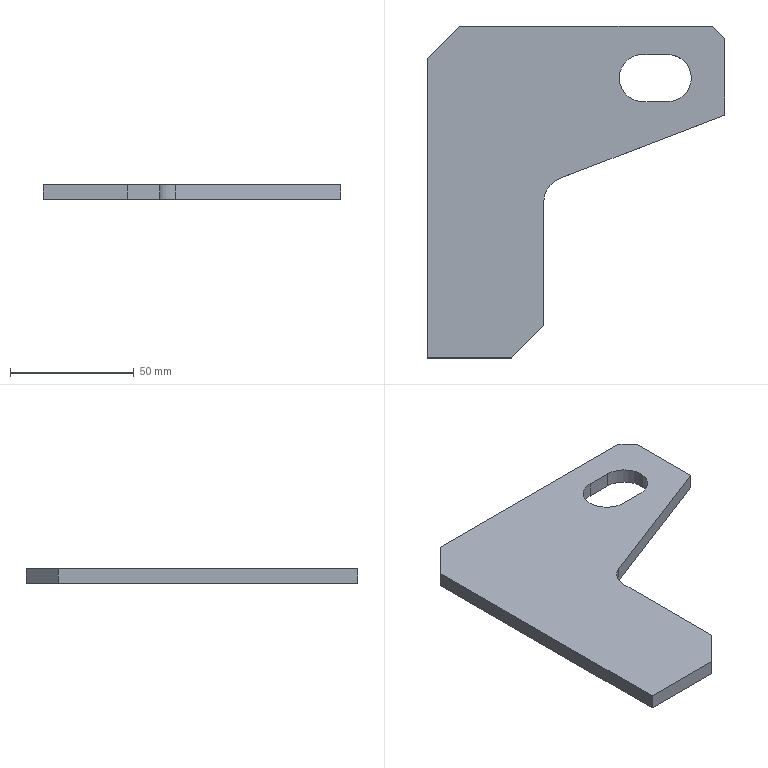Part | STEP file | 筋Plate-200×100-5-1 | 1 solid | 17 faces | box 120 x 134 x 6 mm | volume 55809 mm3 | plane 13 | cylinder 4 | commonest cylinder face diameters 19 x3 20 x1
STEP:
#1=CARTESIAN_POINT('',(0.,0.,0.));
#2=DIRECTION('',(0.,0.,1.));
#3=DIRECTION('',(1.,0.,0.));
#4=AXIS2_PLACEMENT_3D('',#1,#2,#3);
#5=CARTESIAN_POINT('',(27.,80.5,3.));
#6=VERTEX_POINT('',#5);
#7=CARTESIAN_POINT('',(27.,80.5,-3.));
#8=VERTEX_POINT('',#7);
#9=CARTESIAN_POINT('',(27.,80.5,-3.));
#10=DIRECTION('',(0.,0.,-1.));
#11=VECTOR('',#10,1.);
#12=LINE('',#9,#11);
#13=CARTESIAN_POINT('',(27.,71.,-3.));
#14=DIRECTION('',(0.,0.,-1.));
#15=DIRECTION('',(-1.,0.,0.));
#16=AXIS2_PLACEMENT_3D('',#13,#14,#15);
#17=CYLINDRICAL_SURFACE('',#16,9.5);
#18=CARTESIAN_POINT('',(1.571,0.));
#19=DIRECTION('',(0.,1.));
#20=VECTOR('',#19,1.);
#21=LINE('',#18,#20);
#22=(GEOMETRIC_REPRESENTATION_CONTEXT(2)PARAMETRIC_REPRESENTATION_CONTEXT()REPRESENTATION_CONTEXT('',''));
#23=DEFINITIONAL_REPRESENTATION('',(#21),#22);
#24=PCURVE('',#17,#23);
#25=CARTESIAN_POINT('',(37.,80.5,-3.));
#26=DIRECTION('',(0.,1.,0.));
#27=DIRECTION('',(0.,0.,1.));
#28=AXIS2_PLACEMENT_3D('',#25,#26,#27);
#29=PLANE('',#28);
#30=CARTESIAN_POINT('',(0.,-10.));
#31=DIRECTION('',(-1.,0.));
#32=VECTOR('',#31,1.);
#33=LINE('',#30,#32);
#34=(GEOMETRIC_REPRESENTATION_CONTEXT(2)PARAMETRIC_REPRESENTATION_CONTEXT()REPRESENTATION_CONTEXT('',''));
#35=DEFINITIONAL_REPRESENTATION('',(#33),#34);
#36=PCURVE('',#29,#35);
#37=SURFACE_CURVE('',#12,(#24,#36),.PCURVE_S1.);
#38=EDGE_CURVE('',#6,#8,#37,.T.);
#39=ORIENTED_EDGE('',*,*,#38,.T.);
#40=CARTESIAN_POINT('',(17.5,71.,-3.));
#41=VERTEX_POINT('',#40);
#42=CARTESIAN_POINT('',(27.,71.,-3.));
#43=DIRECTION('',(0.,0.,-1.));
#44=DIRECTION('',(-1.,0.,0.));
#45=AXIS2_PLACEMENT_3D('',#42,#43,#44);
#46=CIRCLE('',#45,9.5);
#47=CARTESIAN_POINT('',(0.,0.));
#48=DIRECTION('',(1.,0.));
#49=VECTOR('',#48,1.);
#50=LINE('',#47,#49);
#51=(GEOMETRIC_REPRESENTATION_CONTEXT(2)PARAMETRIC_REPRESENTATION_CONTEXT()REPRESENTATION_CONTEXT('',''));
#52=DEFINITIONAL_REPRESENTATION('',(#50),#51);
#53=PCURVE('',#17,#52);
#54=CARTESIAN_POINT('',(0.,0.,-3.));
#55=DIRECTION('',(0.,0.,1.));
#56=DIRECTION('',(1.,0.,0.));
#57=AXIS2_PLACEMENT_3D('',#54,#55,#56);
#58=PLANE('',#57);
#59=CARTESIAN_POINT('',(17.5,71.));
#60=CARTESIAN_POINT('',(17.5,87.454));
#61=CARTESIAN_POINT('',(31.75,79.227));
#62=CARTESIAN_POINT('',(46.,71.));
#63=CARTESIAN_POINT('',(31.75,62.773));
#64=CARTESIAN_POINT('',(17.5,54.546));
#65=CARTESIAN_POINT('',(17.5,71.));
#66=(BOUNDED_CURVE()B_SPLINE_CURVE(2,(#59,#60,#61,#62,#63,#64,#65),.UNSPECIFIED.,.T.,.F.)B_SPLINE_CURVE_WITH_KNOTS((1,2,2,2,2,1),(-2.094,0.,2.094,4.189,6.283,8.378),.UNSPECIFIED.)CURVE()GEOMETRIC_REPRESENTATION_ITEM()RATIONAL_B_SPLINE_CURVE((1.,0.5,1.,0.5,1.,0.5,1.))REPRESENTATION_ITEM(''));
#67=(GEOMETRIC_REPRESENTATION_CONTEXT(2)PARAMETRIC_REPRESENTATION_CONTEXT()REPRESENTATION_CONTEXT('',''));
#68=DEFINITIONAL_REPRESENTATION('',(#66),#67);
#69=PCURVE('',#58,#68);
#70=SURFACE_CURVE('',#46,(#53,#69),.PCURVE_S1.);
#71=EDGE_CURVE('',#41,#8,#70,.T.);
#72=ORIENTED_EDGE('',*,*,#71,.F.);
#73=CARTESIAN_POINT('',(17.5,71.,3.));
#74=VERTEX_POINT('',#73);
#75=CARTESIAN_POINT('',(17.5,71.,-3.));
#76=DIRECTION('',(0.,0.,-1.));
#77=VECTOR('',#76,1.);
#78=LINE('',#75,#77);
#79=CARTESIAN_POINT('',(0.,0.));
#80=DIRECTION('',(0.,1.));
#81=VECTOR('',#80,1.);
#82=LINE('',#79,#81);
#83=(GEOMETRIC_REPRESENTATION_CONTEXT(2)PARAMETRIC_REPRESENTATION_CONTEXT()REPRESENTATION_CONTEXT('',''));
#84=DEFINITIONAL_REPRESENTATION('',(#82),#83);
#85=PCURVE('',#17,#84);
#86=CARTESIAN_POINT('',(27.,71.,-3.));
#87=DIRECTION('',(0.,0.,-1.));
#88=DIRECTION('',(-1.,0.,0.));
#89=AXIS2_PLACEMENT_3D('',#86,#87,#88);
#90=CYLINDRICAL_SURFACE('',#89,9.5);
#91=CARTESIAN_POINT('',(6.283,0.));
#92=DIRECTION('',(0.,1.));
#93=VECTOR('',#92,1.);
#94=LINE('',#91,#93);
#95=(GEOMETRIC_REPRESENTATION_CONTEXT(2)PARAMETRIC_REPRESENTATION_CONTEXT()REPRESENTATION_CONTEXT('',''));
#96=DEFINITIONAL_REPRESENTATION('',(#94),#95);
#97=PCURVE('',#90,#96);
#98=SURFACE_CURVE('',#78,(#85,#97),.PCURVE_S1.);
#99=EDGE_CURVE('',#74,#41,#98,.T.);
#100=ORIENTED_EDGE('',*,*,#99,.F.);
#101=CARTESIAN_POINT('',(27.,71.,3.));
#102=DIRECTION('',(0.,0.,1.));
#103=DIRECTION('',(1.,0.,0.));
#104=AXIS2_PLACEMENT_3D('',#101,#102,#103);
#105=CIRCLE('',#104,9.5);
#106=CARTESIAN_POINT('',(3.142,-6.));
#107=DIRECTION('',(-1.,0.));
#108=VECTOR('',#107,1.);
#109=LINE('',#106,#108);
#110=(GEOMETRIC_REPRESENTATION_CONTEXT(2)PARAMETRIC_REPRESENTATION_CONTEXT()REPRESENTATION_CONTEXT('',''));
#111=DEFINITIONAL_REPRESENTATION('',(#109),#110);
#112=PCURVE('',#17,#111);
#113=CARTESIAN_POINT('',(0.,0.,3.));
#114=DIRECTION('',(0.,0.,1.));
#115=DIRECTION('',(1.,0.,0.));
#116=AXIS2_PLACEMENT_3D('',#113,#114,#115);
#117=PLANE('',#116);
#118=CARTESIAN_POINT('',(27.,71.));
#119=DIRECTION('',(1.,0.));
#120=AXIS2_PLACEMENT_2D('',#118,#119);
#121=CIRCLE('',#120,9.5);
#122=(GEOMETRIC_REPRESENTATION_CONTEXT(2)PARAMETRIC_REPRESENTATION_CONTEXT()REPRESENTATION_CONTEXT('',''));
#123=DEFINITIONAL_REPRESENTATION('',(#121),#122);
#124=PCURVE('',#117,#123);
#125=SURFACE_CURVE('',#105,(#112,#124),.PCURVE_S1.);
#126=EDGE_CURVE('',#6,#74,#125,.T.);
#127=ORIENTED_EDGE('',*,*,#126,.F.);
#128=EDGE_LOOP('',(#39,#72,#100,#127));
#129=FACE_BOUND('',#128,.F.);
#130=ADVANCED_FACE('',(#129),#17,.F.);
#131=CARTESIAN_POINT('',(55.,92.,-3.));
#132=VERTEX_POINT('',#131);
#133=CARTESIAN_POINT('',(-47.,92.,-3.));
#134=VERTEX_POINT('',#133);
#135=CARTESIAN_POINT('',(-60.,92.,-3.));
#136=DIRECTION('',(-1.,0.,0.));
#137=VECTOR('',#136,1.);
#138=LINE('',#135,#137);
#139=CARTESIAN_POINT('',(-60.,92.));
#140=DIRECTION('',(-1.,0.));
#141=VECTOR('',#140,1.);
#142=LINE('',#139,#141);
#143=(GEOMETRIC_REPRESENTATION_CONTEXT(2)PARAMETRIC_REPRESENTATION_CONTEXT()REPRESENTATION_CONTEXT('',''));
#144=DEFINITIONAL_REPRESENTATION('',(#142),#143);
#145=PCURVE('',#58,#144);
#146=CARTESIAN_POINT('',(-60.,92.,3.));
#147=DIRECTION('',(0.,-1.,0.));
#148=DIRECTION('',(0.,0.,-1.));
#149=AXIS2_PLACEMENT_3D('',#146,#147,#148);
#150=PLANE('',#149);
#151=CARTESIAN_POINT('',(6.,0.));
#152=DIRECTION('',(0.,-1.));
#153=VECTOR('',#152,1.);
#154=LINE('',#151,#153);
#155=(GEOMETRIC_REPRESENTATION_CONTEXT(2)PARAMETRIC_REPRESENTATION_CONTEXT()REPRESENTATION_CONTEXT('',''));
#156=DEFINITIONAL_REPRESENTATION('',(#154),#155);
#157=PCURVE('',#150,#156);
#158=SURFACE_CURVE('',#138,(#145,#157),.PCURVE_S1.);
#159=EDGE_CURVE('',#132,#134,#158,.T.);
#160=ORIENTED_EDGE('',*,*,#159,.F.);
#161=CARTESIAN_POINT('',(60.,87.,-3.));
#162=VERTEX_POINT('',#161);
#163=CARTESIAN_POINT('',(55.,92.,-3.));
#164=DIRECTION('',(0.7071,-0.7071,0.));
#165=VECTOR('',#164,1.);
#166=LINE('',#163,#165);
#167=CARTESIAN_POINT('',(55.,92.));
#168=DIRECTION('',(0.7071,-0.7071));
#169=VECTOR('',#168,1.);
#170=LINE('',#167,#169);
#171=(GEOMETRIC_REPRESENTATION_CONTEXT(2)PARAMETRIC_REPRESENTATION_CONTEXT()REPRESENTATION_CONTEXT('',''));
#172=DEFINITIONAL_REPRESENTATION('',(#170),#171);
#173=PCURVE('',#58,#172);
#174=CARTESIAN_POINT('',(55.,92.,3.));
#175=DIRECTION('',(-0.7071,-0.7071,0.));
#176=DIRECTION('',(0.,0.,-1.));
#177=AXIS2_PLACEMENT_3D('',#174,#175,#176);
#178=PLANE('',#177);
#179=CARTESIAN_POINT('',(6.,0.));
#180=DIRECTION('',(0.,1.));
#181=VECTOR('',#180,1.);
#182=LINE('',#179,#181);
#183=(GEOMETRIC_REPRESENTATION_CONTEXT(2)PARAMETRIC_REPRESENTATION_CONTEXT()REPRESENTATION_CONTEXT('',''));
#184=DEFINITIONAL_REPRESENTATION('',(#182),#183);
#185=PCURVE('',#178,#184);
#186=SURFACE_CURVE('',#166,(#173,#185),.PCURVE_S1.);
#187=EDGE_CURVE('',#132,#162,#186,.T.);
#188=ORIENTED_EDGE('',*,*,#187,.T.);
#189=CARTESIAN_POINT('',(60.,56.,-3.));
#190=VERTEX_POINT('',#189);
#191=CARTESIAN_POINT('',(60.,92.,-3.));
#192=DIRECTION('',(0.,1.,0.));
#193=VECTOR('',#192,1.);
#194=LINE('',#191,#193);
#195=CARTESIAN_POINT('',(60.,92.));
#196=DIRECTION('',(0.,1.));
#197=VECTOR('',#196,1.);
#198=LINE('',#195,#197);
#199=(GEOMETRIC_REPRESENTATION_CONTEXT(2)PARAMETRIC_REPRESENTATION_CONTEXT()REPRESENTATION_CONTEXT('',''));
#200=DEFINITIONAL_REPRESENTATION('',(#198),#199);
#201=PCURVE('',#58,#200);
#202=CARTESIAN_POINT('',(60.,92.,3.));
#203=DIRECTION('',(-1.,0.,0.));
#204=DIRECTION('',(0.,-1.,0.));
#205=AXIS2_PLACEMENT_3D('',#202,#203,#204);
#206=PLANE('',#205);
#207=CARTESIAN_POINT('',(0.,-6.));
#208=DIRECTION('',(-1.,0.));
#209=VECTOR('',#208,1.);
#210=LINE('',#207,#209);
#211=(GEOMETRIC_REPRESENTATION_CONTEXT(2)PARAMETRIC_REPRESENTATION_CONTEXT()REPRESENTATION_CONTEXT('',''));
#212=DEFINITIONAL_REPRESENTATION('',(#210),#211);
#213=PCURVE('',#206,#212);
#214=SURFACE_CURVE('',#194,(#201,#213),.PCURVE_S1.);
#215=EDGE_CURVE('',#190,#162,#214,.T.);
#216=ORIENTED_EDGE('',*,*,#215,.F.);
#217=CARTESIAN_POINT('',(-6.581,30.462,-3.));
#218=VERTEX_POINT('',#217);
#219=CARTESIAN_POINT('',(60.,56.,-3.));
#220=DIRECTION('',(-0.9337,-0.3581,0.));
#221=VECTOR('',#220,1.);
#222=LINE('',#219,#221);
#223=CARTESIAN_POINT('',(60.,56.));
#224=DIRECTION('',(-0.9337,-0.3581));
#225=VECTOR('',#224,1.);
#226=LINE('',#223,#225);
#227=(GEOMETRIC_REPRESENTATION_CONTEXT(2)PARAMETRIC_REPRESENTATION_CONTEXT()REPRESENTATION_CONTEXT('',''));
#228=DEFINITIONAL_REPRESENTATION('',(#226),#227);
#229=PCURVE('',#58,#228);
#230=CARTESIAN_POINT('',(60.,56.,-3.));
#231=DIRECTION('',(-0.3581,0.9337,0.));
#232=DIRECTION('',(-0.9337,-0.3581,0.));
#233=AXIS2_PLACEMENT_3D('',#230,#231,#232);
#234=PLANE('',#233);
#235=CARTESIAN_POINT('',(0.,0.));
#236=DIRECTION('',(1.,0.));
#237=VECTOR('',#236,1.);
#238=LINE('',#235,#237);
#239=(GEOMETRIC_REPRESENTATION_CONTEXT(2)PARAMETRIC_REPRESENTATION_CONTEXT()REPRESENTATION_CONTEXT('',''));
#240=DEFINITIONAL_REPRESENTATION('',(#238),#239);
#241=PCURVE('',#234,#240);
#242=SURFACE_CURVE('',#222,(#229,#241),.PCURVE_S1.);
#243=EDGE_CURVE('',#190,#218,#242,.T.);
#244=ORIENTED_EDGE('',*,*,#243,.T.);
#245=CARTESIAN_POINT('',(-13.,21.125,-3.));
#246=VERTEX_POINT('',#245);
#247=CARTESIAN_POINT('',(-3.,21.125,-3.));
#248=DIRECTION('',(0.,0.,1.));
#249=DIRECTION('',(1.,0.,0.));
#250=AXIS2_PLACEMENT_3D('',#247,#248,#249);
#251=CIRCLE('',#250,10.);
#252=CARTESIAN_POINT('',(-3.,21.125));
#253=DIRECTION('',(1.,0.));
#254=AXIS2_PLACEMENT_2D('',#252,#253);
#255=CIRCLE('',#254,10.);
#256=(GEOMETRIC_REPRESENTATION_CONTEXT(2)PARAMETRIC_REPRESENTATION_CONTEXT()REPRESENTATION_CONTEXT('',''));
#257=DEFINITIONAL_REPRESENTATION('',(#255),#256);
#258=PCURVE('',#58,#257);
#259=CARTESIAN_POINT('',(-3.,21.125,-3.));
#260=DIRECTION('',(0.,0.,-1.));
#261=DIRECTION('',(-1.,0.,0.));
#262=AXIS2_PLACEMENT_3D('',#259,#260,#261);
#263=CYLINDRICAL_SURFACE('',#262,10.);
#264=CARTESIAN_POINT('',(3.142,0.));
#265=DIRECTION('',(-1.,0.));
#266=VECTOR('',#265,1.);
#267=LINE('',#264,#266);
#268=(GEOMETRIC_REPRESENTATION_CONTEXT(2)PARAMETRIC_REPRESENTATION_CONTEXT()REPRESENTATION_CONTEXT('',''));
#269=DEFINITIONAL_REPRESENTATION('',(#267),#268);
#270=PCURVE('',#263,#269);
#271=SURFACE_CURVE('',#251,(#258,#270),.PCURVE_S1.);
#272=EDGE_CURVE('',#218,#246,#271,.T.);
#273=ORIENTED_EDGE('',*,*,#272,.T.);
#274=CARTESIAN_POINT('',(-13.,-29.,-3.));
#275=VERTEX_POINT('',#274);
#276=CARTESIAN_POINT('',(-13.,-92.,-3.));
#277=DIRECTION('',(0.,-1.,0.));
#278=VECTOR('',#277,1.);
#279=LINE('',#276,#278);
#280=CARTESIAN_POINT('',(-13.,-92.));
#281=DIRECTION('',(0.,-1.));
#282=VECTOR('',#281,1.);
#283=LINE('',#280,#282);
#284=(GEOMETRIC_REPRESENTATION_CONTEXT(2)PARAMETRIC_REPRESENTATION_CONTEXT()REPRESENTATION_CONTEXT('',''));
#285=DEFINITIONAL_REPRESENTATION('',(#283),#284);
#286=PCURVE('',#58,#285);
#287=CARTESIAN_POINT('',(-13.,-92.,-3.));
#288=DIRECTION('',(-1.,0.,0.));
#289=DIRECTION('',(0.,-1.,0.));
#290=AXIS2_PLACEMENT_3D('',#287,#288,#289);
#291=PLANE('',#290);
#292=CARTESIAN_POINT('',(0.,0.));
#293=DIRECTION('',(1.,0.));
#294=VECTOR('',#293,1.);
#295=LINE('',#292,#294);
#296=(GEOMETRIC_REPRESENTATION_CONTEXT(2)PARAMETRIC_REPRESENTATION_CONTEXT()REPRESENTATION_CONTEXT('',''));
#297=DEFINITIONAL_REPRESENTATION('',(#295),#296);
#298=PCURVE('',#291,#297);
#299=SURFACE_CURVE('',#279,(#286,#298),.PCURVE_S1.);
#300=EDGE_CURVE('',#246,#275,#299,.T.);
#301=ORIENTED_EDGE('',*,*,#300,.T.);
#302=CARTESIAN_POINT('',(-26.,-42.,-3.));
#303=VERTEX_POINT('',#302);
#304=CARTESIAN_POINT('',(-26.,-42.,-3.));
#305=DIRECTION('',(-0.7071,-0.7071,0.));
#306=VECTOR('',#305,1.);
#307=LINE('',#304,#306);
#308=CARTESIAN_POINT('',(-26.,-42.));
#309=DIRECTION('',(-0.7071,-0.7071));
#310=VECTOR('',#309,1.);
#311=LINE('',#308,#310);
#312=(GEOMETRIC_REPRESENTATION_CONTEXT(2)PARAMETRIC_REPRESENTATION_CONTEXT()REPRESENTATION_CONTEXT('',''));
#313=DEFINITIONAL_REPRESENTATION('',(#311),#312);
#314=PCURVE('',#58,#313);
#315=CARTESIAN_POINT('',(-26.,-42.,3.));
#316=DIRECTION('',(-0.7071,0.7071,0.));
#317=DIRECTION('',(0.,0.,1.));
#318=AXIS2_PLACEMENT_3D('',#315,#316,#317);
#319=PLANE('',#318);
#320=CARTESIAN_POINT('',(-6.,0.));
#321=DIRECTION('',(0.,-1.));
#322=VECTOR('',#321,1.);
#323=LINE('',#320,#322);
#324=(GEOMETRIC_REPRESENTATION_CONTEXT(2)PARAMETRIC_REPRESENTATION_CONTEXT()REPRESENTATION_CONTEXT('',''));
#325=DEFINITIONAL_REPRESENTATION('',(#323),#324);
#326=PCURVE('',#319,#325);
#327=SURFACE_CURVE('',#307,(#314,#326),.PCURVE_S1.);
#328=EDGE_CURVE('',#275,#303,#327,.T.);
#329=ORIENTED_EDGE('',*,*,#328,.T.);
#330=CARTESIAN_POINT('',(-60.,-42.,-3.));
#331=VERTEX_POINT('',#330);
#332=CARTESIAN_POINT('',(-60.,-42.,-3.));
#333=DIRECTION('',(1.,0.,0.));
#334=VECTOR('',#333,1.);
#335=LINE('',#332,#334);
#336=CARTESIAN_POINT('',(-60.,-42.));
#337=DIRECTION('',(1.,0.));
#338=VECTOR('',#337,1.);
#339=LINE('',#336,#338);
#340=(GEOMETRIC_REPRESENTATION_CONTEXT(2)PARAMETRIC_REPRESENTATION_CONTEXT()REPRESENTATION_CONTEXT('',''));
#341=DEFINITIONAL_REPRESENTATION('',(#339),#340);
#342=PCURVE('',#58,#341);
#343=CARTESIAN_POINT('',(-60.,-42.,3.));
#344=DIRECTION('',(0.,1.,0.));
#345=DIRECTION('',(0.,0.,1.));
#346=AXIS2_PLACEMENT_3D('',#343,#344,#345);
#347=PLANE('',#346);
#348=CARTESIAN_POINT('',(-6.,0.));
#349=DIRECTION('',(0.,1.));
#350=VECTOR('',#349,1.);
#351=LINE('',#348,#350);
#352=(GEOMETRIC_REPRESENTATION_CONTEXT(2)PARAMETRIC_REPRESENTATION_CONTEXT()REPRESENTATION_CONTEXT('',''));
#353=DEFINITIONAL_REPRESENTATION('',(#351),#352);
#354=PCURVE('',#347,#353);
#355=SURFACE_CURVE('',#335,(#342,#354),.PCURVE_S1.);
#356=EDGE_CURVE('',#331,#303,#355,.T.);
#357=ORIENTED_EDGE('',*,*,#356,.F.);
#358=CARTESIAN_POINT('',(-60.,79.,-3.));
#359=VERTEX_POINT('',#358);
#360=CARTESIAN_POINT('',(-60.,92.,-3.));
#361=DIRECTION('',(0.,-1.,0.));
#362=VECTOR('',#361,1.);
#363=LINE('',#360,#362);
#364=CARTESIAN_POINT('',(-60.,92.));
#365=DIRECTION('',(0.,-1.));
#366=VECTOR('',#365,1.);
#367=LINE('',#364,#366);
#368=(GEOMETRIC_REPRESENTATION_CONTEXT(2)PARAMETRIC_REPRESENTATION_CONTEXT()REPRESENTATION_CONTEXT('',''));
#369=DEFINITIONAL_REPRESENTATION('',(#367),#368);
#370=PCURVE('',#58,#369);
#371=CARTESIAN_POINT('',(-60.,92.,3.));
#372=DIRECTION('',(1.,0.,0.));
#373=DIRECTION('',(0.,1.,0.));
#374=AXIS2_PLACEMENT_3D('',#371,#372,#373);
#375=PLANE('',#374);
#376=CARTESIAN_POINT('',(0.,-6.));
#377=DIRECTION('',(-1.,0.));
#378=VECTOR('',#377,1.);
#379=LINE('',#376,#378);
#380=(GEOMETRIC_REPRESENTATION_CONTEXT(2)PARAMETRIC_REPRESENTATION_CONTEXT()REPRESENTATION_CONTEXT('',''));
#381=DEFINITIONAL_REPRESENTATION('',(#379),#380);
#382=PCURVE('',#375,#381);
#383=SURFACE_CURVE('',#363,(#370,#382),.PCURVE_S1.);
#384=EDGE_CURVE('',#359,#331,#383,.T.);
#385=ORIENTED_EDGE('',*,*,#384,.F.);
#386=CARTESIAN_POINT('',(-60.,79.,-3.));
#387=DIRECTION('',(0.7071,0.7071,0.));
#388=VECTOR('',#387,1.);
#389=LINE('',#386,#388);
#390=CARTESIAN_POINT('',(-60.,79.));
#391=DIRECTION('',(0.7071,0.7071));
#392=VECTOR('',#391,1.);
#393=LINE('',#390,#392);
#394=(GEOMETRIC_REPRESENTATION_CONTEXT(2)PARAMETRIC_REPRESENTATION_CONTEXT()REPRESENTATION_CONTEXT('',''));
#395=DEFINITIONAL_REPRESENTATION('',(#393),#394);
#396=PCURVE('',#58,#395);
#397=CARTESIAN_POINT('',(-60.,79.,3.));
#398=DIRECTION('',(0.7071,-0.7071,0.));
#399=DIRECTION('',(0.,0.,-1.));
#400=AXIS2_PLACEMENT_3D('',#397,#398,#399);
#401=PLANE('',#400);
#402=CARTESIAN_POINT('',(6.,0.));
#403=DIRECTION('',(0.,1.));
#404=VECTOR('',#403,1.);
#405=LINE('',#402,#404);
#406=(GEOMETRIC_REPRESENTATION_CONTEXT(2)PARAMETRIC_REPRESENTATION_CONTEXT()REPRESENTATION_CONTEXT('',''));
#407=DEFINITIONAL_REPRESENTATION('',(#405),#406);
#408=PCURVE('',#401,#407);
#409=SURFACE_CURVE('',#389,(#396,#408),.PCURVE_S1.);
#410=EDGE_CURVE('',#359,#134,#409,.T.);
#411=ORIENTED_EDGE('',*,*,#410,.T.);
#412=EDGE_LOOP('',(#160,#188,#216,#244,#273,#301,#329,#357,#385,#411));
#413=FACE_BOUND('',#412,.T.);
#414=CARTESIAN_POINT('',(37.,80.5,-3.));
#415=VERTEX_POINT('',#414);
#416=CARTESIAN_POINT('',(37.,61.5,-3.));
#417=VERTEX_POINT('',#416);
#418=CARTESIAN_POINT('',(37.,71.,-3.));
#419=DIRECTION('',(0.,0.,-1.));
#420=DIRECTION('',(-1.,0.,0.));
#421=AXIS2_PLACEMENT_3D('',#418,#419,#420);
#422=CIRCLE('',#421,9.5);
#423=CARTESIAN_POINT('',(27.5,71.));
#424=CARTESIAN_POINT('',(27.5,87.454));
#425=CARTESIAN_POINT('',(41.75,79.227));
#426=CARTESIAN_POINT('',(56.,71.));
#427=CARTESIAN_POINT('',(41.75,62.773));
#428=CARTESIAN_POINT('',(27.5,54.546));
#429=CARTESIAN_POINT('',(27.5,71.));
#430=(BOUNDED_CURVE()B_SPLINE_CURVE(2,(#423,#424,#425,#426,#427,#428,#429),.UNSPECIFIED.,.T.,.F.)B_SPLINE_CURVE_WITH_KNOTS((1,2,2,2,2,1),(-2.094,0.,2.094,4.189,6.283,8.378),.UNSPECIFIED.)CURVE()GEOMETRIC_REPRESENTATION_ITEM()RATIONAL_B_SPLINE_CURVE((1.,0.5,1.,0.5,1.,0.5,1.))REPRESENTATION_ITEM(''));
#431=(GEOMETRIC_REPRESENTATION_CONTEXT(2)PARAMETRIC_REPRESENTATION_CONTEXT()REPRESENTATION_CONTEXT('',''));
#432=DEFINITIONAL_REPRESENTATION('',(#430),#431);
#433=PCURVE('',#58,#432);
#434=CARTESIAN_POINT('',(37.,71.,-3.));
#435=DIRECTION('',(0.,0.,-1.));
#436=DIRECTION('',(-1.,0.,0.));
#437=AXIS2_PLACEMENT_3D('',#434,#435,#436);
#438=CYLINDRICAL_SURFACE('',#437,9.5);
#439=CARTESIAN_POINT('',(0.,0.));
#440=DIRECTION('',(1.,0.));
#441=VECTOR('',#440,1.);
#442=LINE('',#439,#441);
#443=(GEOMETRIC_REPRESENTATION_CONTEXT(2)PARAMETRIC_REPRESENTATION_CONTEXT()REPRESENTATION_CONTEXT('',''));
#444=DEFINITIONAL_REPRESENTATION('',(#442),#443);
#445=PCURVE('',#438,#444);
#446=SURFACE_CURVE('',#422,(#433,#445),.PCURVE_S1.);
#447=EDGE_CURVE('',#415,#417,#446,.T.);
#448=ORIENTED_EDGE('',*,*,#447,.F.);
#449=CARTESIAN_POINT('',(37.,80.5,-3.));
#450=DIRECTION('',(-1.,0.,0.));
#451=VECTOR('',#450,1.);
#452=LINE('',#449,#451);
#453=CARTESIAN_POINT('',(37.,80.5));
#454=DIRECTION('',(-1.,0.));
#455=VECTOR('',#454,1.);
#456=LINE('',#453,#455);
#457=(GEOMETRIC_REPRESENTATION_CONTEXT(2)PARAMETRIC_REPRESENTATION_CONTEXT()REPRESENTATION_CONTEXT('',''));
#458=DEFINITIONAL_REPRESENTATION('',(#456),#457);
#459=PCURVE('',#58,#458);
#460=CARTESIAN_POINT('',(0.,0.));
#461=DIRECTION('',(0.,-1.));
#462=VECTOR('',#461,1.);
#463=LINE('',#460,#462);
#464=(GEOMETRIC_REPRESENTATION_CONTEXT(2)PARAMETRIC_REPRESENTATION_CONTEXT()REPRESENTATION_CONTEXT('',''));
#465=DEFINITIONAL_REPRESENTATION('',(#463),#464);
#466=PCURVE('',#29,#465);
#467=SURFACE_CURVE('',#452,(#459,#466),.PCURVE_S1.);
#468=EDGE_CURVE('',#415,#8,#467,.T.);
#469=ORIENTED_EDGE('',*,*,#468,.T.);
#470=ORIENTED_EDGE('',*,*,#71,.F.);
#471=CARTESIAN_POINT('',(27.,61.5,-3.));
#472=VERTEX_POINT('',#471);
#473=CARTESIAN_POINT('',(27.,71.,-3.));
#474=DIRECTION('',(0.,0.,-1.));
#475=DIRECTION('',(-1.,0.,0.));
#476=AXIS2_PLACEMENT_3D('',#473,#474,#475);
#477=CIRCLE('',#476,9.5);
#478=CARTESIAN_POINT('',(17.5,71.));
#479=CARTESIAN_POINT('',(17.5,87.454));
#480=CARTESIAN_POINT('',(31.75,79.227));
#481=CARTESIAN_POINT('',(46.,71.));
#482=CARTESIAN_POINT('',(31.75,62.773));
#483=CARTESIAN_POINT('',(17.5,54.546));
#484=CARTESIAN_POINT('',(17.5,71.));
#485=(BOUNDED_CURVE()B_SPLINE_CURVE(2,(#478,#479,#480,#481,#482,#483,#484),.UNSPECIFIED.,.T.,.F.)B_SPLINE_CURVE_WITH_KNOTS((1,2,2,2,2,1),(-2.094,0.,2.094,4.189,6.283,8.378),.UNSPECIFIED.)CURVE()GEOMETRIC_REPRESENTATION_ITEM()RATIONAL_B_SPLINE_CURVE((1.,0.5,1.,0.5,1.,0.5,1.))REPRESENTATION_ITEM(''));
#486=(GEOMETRIC_REPRESENTATION_CONTEXT(2)PARAMETRIC_REPRESENTATION_CONTEXT()REPRESENTATION_CONTEXT('',''));
#487=DEFINITIONAL_REPRESENTATION('',(#485),#486);
#488=PCURVE('',#58,#487);
#489=CARTESIAN_POINT('',(0.,0.));
#490=DIRECTION('',(1.,0.));
#491=VECTOR('',#490,1.);
#492=LINE('',#489,#491);
#493=(GEOMETRIC_REPRESENTATION_CONTEXT(2)PARAMETRIC_REPRESENTATION_CONTEXT()REPRESENTATION_CONTEXT('',''));
#494=DEFINITIONAL_REPRESENTATION('',(#492),#493);
#495=PCURVE('',#90,#494);
#496=SURFACE_CURVE('',#477,(#488,#495),.PCURVE_S1.);
#497=EDGE_CURVE('',#472,#41,#496,.T.);
#498=ORIENTED_EDGE('',*,*,#497,.F.);
#499=CARTESIAN_POINT('',(37.,61.5,-3.));
#500=DIRECTION('',(-1.,0.,0.));
#501=VECTOR('',#500,1.);
#502=LINE('',#499,#501);
#503=CARTESIAN_POINT('',(37.,61.5));
#504=DIRECTION('',(-1.,0.));
#505=VECTOR('',#504,1.);
#506=LINE('',#503,#505);
#507=(GEOMETRIC_REPRESENTATION_CONTEXT(2)PARAMETRIC_REPRESENTATION_CONTEXT()REPRESENTATION_CONTEXT('',''));
#508=DEFINITIONAL_REPRESENTATION('',(#506),#507);
#509=PCURVE('',#58,#508);
#510=CARTESIAN_POINT('',(37.,61.5,-3.));
#511=DIRECTION('',(0.,-1.,0.));
#512=DIRECTION('',(0.,0.,-1.));
#513=AXIS2_PLACEMENT_3D('',#510,#511,#512);
#514=PLANE('',#513);
#515=CARTESIAN_POINT('',(0.,0.));
#516=DIRECTION('',(0.,-1.));
#517=VECTOR('',#516,1.);
#518=LINE('',#515,#517);
#519=(GEOMETRIC_REPRESENTATION_CONTEXT(2)PARAMETRIC_REPRESENTATION_CONTEXT()REPRESENTATION_CONTEXT('',''));
#520=DEFINITIONAL_REPRESENTATION('',(#518),#519);
#521=PCURVE('',#514,#520);
#522=SURFACE_CURVE('',#502,(#509,#521),.PCURVE_S1.);
#523=EDGE_CURVE('',#417,#472,#522,.T.);
#524=ORIENTED_EDGE('',*,*,#523,.F.);
#525=EDGE_LOOP('',(#448,#469,#470,#498,#524));
#526=FACE_BOUND('',#525,.T.);
#527=ADVANCED_FACE('',(#413,#526),#58,.F.);
#528=ORIENTED_EDGE('',*,*,#215,.T.);
#529=CARTESIAN_POINT('',(60.,87.,3.));
#530=VERTEX_POINT('',#529);
#531=CARTESIAN_POINT('',(60.,87.,3.));
#532=DIRECTION('',(0.,0.,1.));
#533=VECTOR('',#532,1.);
#534=LINE('',#531,#533);
#535=CARTESIAN_POINT('',(5.,0.));
#536=DIRECTION('',(0.,1.));
#537=VECTOR('',#536,1.);
#538=LINE('',#535,#537);
#539=(GEOMETRIC_REPRESENTATION_CONTEXT(2)PARAMETRIC_REPRESENTATION_CONTEXT()REPRESENTATION_CONTEXT('',''));
#540=DEFINITIONAL_REPRESENTATION('',(#538),#539);
#541=PCURVE('',#206,#540);
#542=CARTESIAN_POINT('',(0.,7.071));
#543=DIRECTION('',(-1.,0.));
#544=VECTOR('',#543,1.);
#545=LINE('',#542,#544);
#546=(GEOMETRIC_REPRESENTATION_CONTEXT(2)PARAMETRIC_REPRESENTATION_CONTEXT()REPRESENTATION_CONTEXT('',''));
#547=DEFINITIONAL_REPRESENTATION('',(#545),#546);
#548=PCURVE('',#178,#547);
#549=SURFACE_CURVE('',#534,(#541,#548),.PCURVE_S1.);
#550=EDGE_CURVE('',#162,#530,#549,.T.);
#551=ORIENTED_EDGE('',*,*,#550,.T.);
#552=CARTESIAN_POINT('',(60.,56.,3.));
#553=VERTEX_POINT('',#552);
#554=CARTESIAN_POINT('',(60.,92.,3.));
#555=DIRECTION('',(0.,1.,0.));
#556=VECTOR('',#555,1.);
#557=LINE('',#554,#556);
#558=CARTESIAN_POINT('',(0.,0.));
#559=DIRECTION('',(-1.,0.));
#560=VECTOR('',#559,1.);
#561=LINE('',#558,#560);
#562=(GEOMETRIC_REPRESENTATION_CONTEXT(2)PARAMETRIC_REPRESENTATION_CONTEXT()REPRESENTATION_CONTEXT('',''));
#563=DEFINITIONAL_REPRESENTATION('',(#561),#562);
#564=PCURVE('',#206,#563);
#565=CARTESIAN_POINT('',(60.,92.));
#566=DIRECTION('',(0.,1.));
#567=VECTOR('',#566,1.);
#568=LINE('',#565,#567);
#569=(GEOMETRIC_REPRESENTATION_CONTEXT(2)PARAMETRIC_REPRESENTATION_CONTEXT()REPRESENTATION_CONTEXT('',''));
#570=DEFINITIONAL_REPRESENTATION('',(#568),#569);
#571=PCURVE('',#117,#570);
#572=SURFACE_CURVE('',#557,(#564,#571),.PCURVE_S1.);
#573=EDGE_CURVE('',#553,#530,#572,.T.);
#574=ORIENTED_EDGE('',*,*,#573,.F.);
#575=CARTESIAN_POINT('',(60.,56.,-3.));
#576=DIRECTION('',(0.,0.,1.));
#577=VECTOR('',#576,1.);
#578=LINE('',#575,#577);
#579=CARTESIAN_POINT('',(36.,-6.));
#580=DIRECTION('',(0.,1.));
#581=VECTOR('',#580,1.);
#582=LINE('',#579,#581);
#583=(GEOMETRIC_REPRESENTATION_CONTEXT(2)PARAMETRIC_REPRESENTATION_CONTEXT()REPRESENTATION_CONTEXT('',''));
#584=DEFINITIONAL_REPRESENTATION('',(#582),#583);
#585=PCURVE('',#206,#584);
#586=CARTESIAN_POINT('',(0.,0.));
#587=DIRECTION('',(0.,1.));
#588=VECTOR('',#587,1.);
#589=LINE('',#586,#588);
#590=(GEOMETRIC_REPRESENTATION_CONTEXT(2)PARAMETRIC_REPRESENTATION_CONTEXT()REPRESENTATION_CONTEXT('',''));
#591=DEFINITIONAL_REPRESENTATION('',(#589),#590);
#592=PCURVE('',#234,#591);
#593=SURFACE_CURVE('',#578,(#585,#592),.PCURVE_S1.);
#594=EDGE_CURVE('',#190,#553,#593,.T.);
#595=ORIENTED_EDGE('',*,*,#594,.F.);
#596=EDGE_LOOP('',(#528,#551,#574,#595));
#597=FACE_BOUND('',#596,.T.);
#598=ADVANCED_FACE('',(#597),#206,.F.);
#599=CARTESIAN_POINT('',(55.,92.,3.));
#600=VERTEX_POINT('',#599);
#601=CARTESIAN_POINT('',(-47.,92.,3.));
#602=VERTEX_POINT('',#601);
#603=CARTESIAN_POINT('',(-60.,92.,3.));
#604=DIRECTION('',(-1.,0.,0.));
#605=VECTOR('',#604,1.);
#606=LINE('',#603,#605);
#607=CARTESIAN_POINT('',(0.,0.));
#608=DIRECTION('',(0.,-1.));
#609=VECTOR('',#608,1.);
#610=LINE('',#607,#609);
#611=(GEOMETRIC_REPRESENTATION_CONTEXT(2)PARAMETRIC_REPRESENTATION_CONTEXT()REPRESENTATION_CONTEXT('',''));
#612=DEFINITIONAL_REPRESENTATION('',(#610),#611);
#613=PCURVE('',#150,#612);
#614=CARTESIAN_POINT('',(-60.,92.));
#615=DIRECTION('',(-1.,0.));
#616=VECTOR('',#615,1.);
#617=LINE('',#614,#616);
#618=(GEOMETRIC_REPRESENTATION_CONTEXT(2)PARAMETRIC_REPRESENTATION_CONTEXT()REPRESENTATION_CONTEXT('',''));
#619=DEFINITIONAL_REPRESENTATION('',(#617),#618);
#620=PCURVE('',#117,#619);
#621=SURFACE_CURVE('',#606,(#613,#620),.PCURVE_S1.);
#622=EDGE_CURVE('',#600,#602,#621,.T.);
#623=ORIENTED_EDGE('',*,*,#622,.F.);
#624=CARTESIAN_POINT('',(55.,92.,3.));
#625=DIRECTION('',(0.,0.,-1.));
#626=VECTOR('',#625,1.);
#627=LINE('',#624,#626);
#628=CARTESIAN_POINT('',(0.,115.));
#629=DIRECTION('',(1.,0.));
#630=VECTOR('',#629,1.);
#631=LINE('',#628,#630);
#632=(GEOMETRIC_REPRESENTATION_CONTEXT(2)PARAMETRIC_REPRESENTATION_CONTEXT()REPRESENTATION_CONTEXT('',''));
#633=DEFINITIONAL_REPRESENTATION('',(#631),#632);
#634=PCURVE('',#150,#633);
#635=CARTESIAN_POINT('',(0.,0.));
#636=DIRECTION('',(1.,0.));
#637=VECTOR('',#636,1.);
#638=LINE('',#635,#637);
#639=(GEOMETRIC_REPRESENTATION_CONTEXT(2)PARAMETRIC_REPRESENTATION_CONTEXT()REPRESENTATION_CONTEXT('',''));
#640=DEFINITIONAL_REPRESENTATION('',(#638),#639);
#641=PCURVE('',#178,#640);
#642=SURFACE_CURVE('',#627,(#634,#641),.PCURVE_S1.);
#643=EDGE_CURVE('',#600,#132,#642,.T.);
#644=ORIENTED_EDGE('',*,*,#643,.T.);
#645=ORIENTED_EDGE('',*,*,#159,.T.);
#646=CARTESIAN_POINT('',(-47.,92.,3.));
#647=DIRECTION('',(0.,0.,1.));
#648=VECTOR('',#647,1.);
#649=LINE('',#646,#648);
#650=CARTESIAN_POINT('',(0.,13.));
#651=DIRECTION('',(-1.,0.));
#652=VECTOR('',#651,1.);
#653=LINE('',#650,#652);
#654=(GEOMETRIC_REPRESENTATION_CONTEXT(2)PARAMETRIC_REPRESENTATION_CONTEXT()REPRESENTATION_CONTEXT('',''));
#655=DEFINITIONAL_REPRESENTATION('',(#653),#654);
#656=PCURVE('',#150,#655);
#657=CARTESIAN_POINT('',(0.,18.385));
#658=DIRECTION('',(-1.,0.));
#659=VECTOR('',#658,1.);
#660=LINE('',#657,#659);
#661=(GEOMETRIC_REPRESENTATION_CONTEXT(2)PARAMETRIC_REPRESENTATION_CONTEXT()REPRESENTATION_CONTEXT('',''));
#662=DEFINITIONAL_REPRESENTATION('',(#660),#661);
#663=PCURVE('',#401,#662);
#664=SURFACE_CURVE('',#649,(#656,#663),.PCURVE_S1.);
#665=EDGE_CURVE('',#134,#602,#664,.T.);
#666=ORIENTED_EDGE('',*,*,#665,.T.);
#667=EDGE_LOOP('',(#623,#644,#645,#666));
#668=FACE_BOUND('',#667,.T.);
#669=ADVANCED_FACE('',(#668),#150,.F.);
#670=CARTESIAN_POINT('',(-60.,79.,3.));
#671=VERTEX_POINT('',#670);
#672=CARTESIAN_POINT('',(-60.,-42.,3.));
#673=VERTEX_POINT('',#672);
#674=CARTESIAN_POINT('',(-60.,92.,3.));
#675=DIRECTION('',(0.,-1.,0.));
#676=VECTOR('',#675,1.);
#677=LINE('',#674,#676);
#678=CARTESIAN_POINT('',(0.,0.));
#679=DIRECTION('',(-1.,0.));
#680=VECTOR('',#679,1.);
#681=LINE('',#678,#680);
#682=(GEOMETRIC_REPRESENTATION_CONTEXT(2)PARAMETRIC_REPRESENTATION_CONTEXT()REPRESENTATION_CONTEXT('',''));
#683=DEFINITIONAL_REPRESENTATION('',(#681),#682);
#684=PCURVE('',#375,#683);
#685=CARTESIAN_POINT('',(-60.,92.));
#686=DIRECTION('',(0.,-1.));
#687=VECTOR('',#686,1.);
#688=LINE('',#685,#687);
#689=(GEOMETRIC_REPRESENTATION_CONTEXT(2)PARAMETRIC_REPRESENTATION_CONTEXT()REPRESENTATION_CONTEXT('',''));
#690=DEFINITIONAL_REPRESENTATION('',(#688),#689);
#691=PCURVE('',#117,#690);
#692=SURFACE_CURVE('',#677,(#684,#691),.PCURVE_S1.);
#693=EDGE_CURVE('',#671,#673,#692,.T.);
#694=ORIENTED_EDGE('',*,*,#693,.F.);
#695=CARTESIAN_POINT('',(-60.,79.,3.));
#696=DIRECTION('',(0.,0.,-1.));
#697=VECTOR('',#696,1.);
#698=LINE('',#695,#697);
#699=CARTESIAN_POINT('',(-13.,0.));
#700=DIRECTION('',(0.,-1.));
#701=VECTOR('',#700,1.);
#702=LINE('',#699,#701);
#703=(GEOMETRIC_REPRESENTATION_CONTEXT(2)PARAMETRIC_REPRESENTATION_CONTEXT()REPRESENTATION_CONTEXT('',''));
#704=DEFINITIONAL_REPRESENTATION('',(#702),#703);
#705=PCURVE('',#375,#704);
#706=CARTESIAN_POINT('',(0.,0.));
#707=DIRECTION('',(1.,0.));
#708=VECTOR('',#707,1.);
#709=LINE('',#706,#708);
#710=(GEOMETRIC_REPRESENTATION_CONTEXT(2)PARAMETRIC_REPRESENTATION_CONTEXT()REPRESENTATION_CONTEXT('',''));
#711=DEFINITIONAL_REPRESENTATION('',(#709),#710);
#712=PCURVE('',#401,#711);
#713=SURFACE_CURVE('',#698,(#705,#712),.PCURVE_S1.);
#714=EDGE_CURVE('',#671,#359,#713,.T.);
#715=ORIENTED_EDGE('',*,*,#714,.T.);
#716=ORIENTED_EDGE('',*,*,#384,.T.);
#717=CARTESIAN_POINT('',(-60.,-42.,3.));
#718=DIRECTION('',(0.,0.,-1.));
#719=VECTOR('',#718,1.);
#720=LINE('',#717,#719);
#721=CARTESIAN_POINT('',(-134.,0.));
#722=DIRECTION('',(0.,-1.));
#723=VECTOR('',#722,1.);
#724=LINE('',#721,#723);
#725=(GEOMETRIC_REPRESENTATION_CONTEXT(2)PARAMETRIC_REPRESENTATION_CONTEXT()REPRESENTATION_CONTEXT('',''));
#726=DEFINITIONAL_REPRESENTATION('',(#724),#725);
#727=PCURVE('',#375,#726);
#728=CARTESIAN_POINT('',(0.,0.));
#729=DIRECTION('',(-1.,0.));
#730=VECTOR('',#729,1.);
#731=LINE('',#728,#730);
#732=(GEOMETRIC_REPRESENTATION_CONTEXT(2)PARAMETRIC_REPRESENTATION_CONTEXT()REPRESENTATION_CONTEXT('',''));
#733=DEFINITIONAL_REPRESENTATION('',(#731),#732);
#734=PCURVE('',#347,#733);
#735=SURFACE_CURVE('',#720,(#727,#734),.PCURVE_S1.);
#736=EDGE_CURVE('',#673,#331,#735,.T.);
#737=ORIENTED_EDGE('',*,*,#736,.F.);
#738=EDGE_LOOP('',(#694,#715,#716,#737));
#739=FACE_BOUND('',#738,.T.);
#740=ADVANCED_FACE('',(#739),#375,.F.);
#741=ORIENTED_EDGE('',*,*,#356,.T.);
#742=CARTESIAN_POINT('',(-26.,-42.,3.));
#743=VERTEX_POINT('',#742);
#744=CARTESIAN_POINT('',(-26.,-42.,3.));
#745=DIRECTION('',(0.,0.,1.));
#746=VECTOR('',#745,1.);
#747=LINE('',#744,#746);
#748=CARTESIAN_POINT('',(0.,34.));
#749=DIRECTION('',(1.,0.));
#750=VECTOR('',#749,1.);
#751=LINE('',#748,#750);
#752=(GEOMETRIC_REPRESENTATION_CONTEXT(2)PARAMETRIC_REPRESENTATION_CONTEXT()REPRESENTATION_CONTEXT('',''));
#753=DEFINITIONAL_REPRESENTATION('',(#751),#752);
#754=PCURVE('',#347,#753);
#755=CARTESIAN_POINT('',(0.,0.));
#756=DIRECTION('',(1.,0.));
#757=VECTOR('',#756,1.);
#758=LINE('',#755,#757);
#759=(GEOMETRIC_REPRESENTATION_CONTEXT(2)PARAMETRIC_REPRESENTATION_CONTEXT()REPRESENTATION_CONTEXT('',''));
#760=DEFINITIONAL_REPRESENTATION('',(#758),#759);
#761=PCURVE('',#319,#760);
#762=SURFACE_CURVE('',#747,(#754,#761),.PCURVE_S1.);
#763=EDGE_CURVE('',#303,#743,#762,.T.);
#764=ORIENTED_EDGE('',*,*,#763,.T.);
#765=CARTESIAN_POINT('',(-60.,-42.,3.));
#766=DIRECTION('',(1.,0.,0.));
#767=VECTOR('',#766,1.);
#768=LINE('',#765,#767);
#769=CARTESIAN_POINT('',(0.,0.));
#770=DIRECTION('',(0.,1.));
#771=VECTOR('',#770,1.);
#772=LINE('',#769,#771);
#773=(GEOMETRIC_REPRESENTATION_CONTEXT(2)PARAMETRIC_REPRESENTATION_CONTEXT()REPRESENTATION_CONTEXT('',''));
#774=DEFINITIONAL_REPRESENTATION('',(#772),#773);
#775=PCURVE('',#347,#774);
#776=CARTESIAN_POINT('',(-60.,-42.));
#777=DIRECTION('',(1.,0.));
#778=VECTOR('',#777,1.);
#779=LINE('',#776,#778);
#780=(GEOMETRIC_REPRESENTATION_CONTEXT(2)PARAMETRIC_REPRESENTATION_CONTEXT()REPRESENTATION_CONTEXT('',''));
#781=DEFINITIONAL_REPRESENTATION('',(#779),#780);
#782=PCURVE('',#117,#781);
#783=SURFACE_CURVE('',#768,(#775,#782),.PCURVE_S1.);
#784=EDGE_CURVE('',#673,#743,#783,.T.);
#785=ORIENTED_EDGE('',*,*,#784,.F.);
#786=ORIENTED_EDGE('',*,*,#736,.T.);
#787=EDGE_LOOP('',(#741,#764,#785,#786));
#788=FACE_BOUND('',#787,.T.);
#789=ADVANCED_FACE('',(#788),#347,.F.);
#790=CARTESIAN_POINT('',(37.,61.5,3.));
#791=VERTEX_POINT('',#790);
#792=CARTESIAN_POINT('',(37.,80.5,3.));
#793=VERTEX_POINT('',#792);
#794=CARTESIAN_POINT('',(37.,71.,3.));
#795=DIRECTION('',(0.,0.,1.));
#796=DIRECTION('',(1.,0.,0.));
#797=AXIS2_PLACEMENT_3D('',#794,#795,#796);
#798=CIRCLE('',#797,9.5);
#799=CARTESIAN_POINT('',(37.,71.));
#800=DIRECTION('',(1.,0.));
#801=AXIS2_PLACEMENT_2D('',#799,#800);
#802=CIRCLE('',#801,9.5);
#803=(GEOMETRIC_REPRESENTATION_CONTEXT(2)PARAMETRIC_REPRESENTATION_CONTEXT()REPRESENTATION_CONTEXT('',''));
#804=DEFINITIONAL_REPRESENTATION('',(#802),#803);
#805=PCURVE('',#117,#804);
#806=CARTESIAN_POINT('',(9.425,-6.));
#807=DIRECTION('',(-1.,0.));
#808=VECTOR('',#807,1.);
#809=LINE('',#806,#808);
#810=(GEOMETRIC_REPRESENTATION_CONTEXT(2)PARAMETRIC_REPRESENTATION_CONTEXT()REPRESENTATION_CONTEXT('',''));
#811=DEFINITIONAL_REPRESENTATION('',(#809),#810);
#812=PCURVE('',#438,#811);
#813=SURFACE_CURVE('',#798,(#805,#812),.PCURVE_S1.);
#814=EDGE_CURVE('',#791,#793,#813,.T.);
#815=ORIENTED_EDGE('',*,*,#814,.F.);
#816=CARTESIAN_POINT('',(27.,61.5,3.));
#817=VERTEX_POINT('',#816);
#818=CARTESIAN_POINT('',(0.,61.5,3.));
#819=DIRECTION('',(1.,0.,0.));
#820=VECTOR('',#819,1.);
#821=LINE('',#818,#820);
#822=CARTESIAN_POINT('',(0.,61.5));
#823=DIRECTION('',(1.,0.));
#824=VECTOR('',#823,1.);
#825=LINE('',#822,#824);
#826=(GEOMETRIC_REPRESENTATION_CONTEXT(2)PARAMETRIC_REPRESENTATION_CONTEXT()REPRESENTATION_CONTEXT('',''));
#827=DEFINITIONAL_REPRESENTATION('',(#825),#826);
#828=PCURVE('',#117,#827);
#829=CARTESIAN_POINT('',(-6.,-37.));
#830=DIRECTION('',(0.,1.));
#831=VECTOR('',#830,1.);
#832=LINE('',#829,#831);
#833=(GEOMETRIC_REPRESENTATION_CONTEXT(2)PARAMETRIC_REPRESENTATION_CONTEXT()REPRESENTATION_CONTEXT('',''));
#834=DEFINITIONAL_REPRESENTATION('',(#832),#833);
#835=PCURVE('',#514,#834);
#836=SURFACE_CURVE('',#821,(#828,#835),.PCURVE_S1.);
#837=EDGE_CURVE('',#817,#791,#836,.T.);
#838=ORIENTED_EDGE('',*,*,#837,.F.);
#839=CARTESIAN_POINT('',(27.,71.,3.));
#840=DIRECTION('',(0.,0.,1.));
#841=DIRECTION('',(1.,0.,0.));
#842=AXIS2_PLACEMENT_3D('',#839,#840,#841);
#843=CIRCLE('',#842,9.5);
#844=CARTESIAN_POINT('',(27.,71.));
#845=DIRECTION('',(1.,0.));
#846=AXIS2_PLACEMENT_2D('',#844,#845);
#847=CIRCLE('',#846,9.5);
#848=(GEOMETRIC_REPRESENTATION_CONTEXT(2)PARAMETRIC_REPRESENTATION_CONTEXT()REPRESENTATION_CONTEXT('',''));
#849=DEFINITIONAL_REPRESENTATION('',(#847),#848);
#850=PCURVE('',#117,#849);
#851=CARTESIAN_POINT('',(9.425,-6.));
#852=DIRECTION('',(-1.,0.));
#853=VECTOR('',#852,1.);
#854=LINE('',#851,#853);
#855=(GEOMETRIC_REPRESENTATION_CONTEXT(2)PARAMETRIC_REPRESENTATION_CONTEXT()REPRESENTATION_CONTEXT('',''));
#856=DEFINITIONAL_REPRESENTATION('',(#854),#855);
#857=PCURVE('',#90,#856);
#858=SURFACE_CURVE('',#843,(#850,#857),.PCURVE_S1.);
#859=EDGE_CURVE('',#74,#817,#858,.T.);
#860=ORIENTED_EDGE('',*,*,#859,.F.);
#861=ORIENTED_EDGE('',*,*,#126,.F.);
#862=CARTESIAN_POINT('',(0.,80.5,3.));
#863=DIRECTION('',(-1.,0.,0.));
#864=VECTOR('',#863,1.);
#865=LINE('',#862,#864);
#866=CARTESIAN_POINT('',(0.,80.5));
#867=DIRECTION('',(-1.,0.));
#868=VECTOR('',#867,1.);
#869=LINE('',#866,#868);
#870=(GEOMETRIC_REPRESENTATION_CONTEXT(2)PARAMETRIC_REPRESENTATION_CONTEXT()REPRESENTATION_CONTEXT('',''));
#871=DEFINITIONAL_REPRESENTATION('',(#869),#870);
#872=PCURVE('',#117,#871);
#873=CARTESIAN_POINT('',(6.,-37.));
#874=DIRECTION('',(0.,-1.));
#875=VECTOR('',#874,1.);
#876=LINE('',#873,#875);
#877=(GEOMETRIC_REPRESENTATION_CONTEXT(2)PARAMETRIC_REPRESENTATION_CONTEXT()REPRESENTATION_CONTEXT('',''));
#878=DEFINITIONAL_REPRESENTATION('',(#876),#877);
#879=PCURVE('',#29,#878);
#880=SURFACE_CURVE('',#865,(#872,#879),.PCURVE_S1.);
#881=EDGE_CURVE('',#793,#6,#880,.T.);
#882=ORIENTED_EDGE('',*,*,#881,.F.);
#883=EDGE_LOOP('',(#815,#838,#860,#861,#882));
#884=FACE_BOUND('',#883,.T.);
#885=ORIENTED_EDGE('',*,*,#573,.T.);
#886=CARTESIAN_POINT('',(73.5,73.5,3.));
#887=DIRECTION('',(-0.7071,0.7071,0.));
#888=VECTOR('',#887,1.);
#889=LINE('',#886,#888);
#890=CARTESIAN_POINT('',(73.5,73.5));
#891=DIRECTION('',(-0.7071,0.7071));
#892=VECTOR('',#891,1.);
#893=LINE('',#890,#892);
#894=(GEOMETRIC_REPRESENTATION_CONTEXT(2)PARAMETRIC_REPRESENTATION_CONTEXT()REPRESENTATION_CONTEXT('',''));
#895=DEFINITIONAL_REPRESENTATION('',(#893),#894);
#896=PCURVE('',#117,#895);
#897=CARTESIAN_POINT('',(0.,26.163));
#898=DIRECTION('',(0.,-1.));
#899=VECTOR('',#898,1.);
#900=LINE('',#897,#899);
#901=(GEOMETRIC_REPRESENTATION_CONTEXT(2)PARAMETRIC_REPRESENTATION_CONTEXT()REPRESENTATION_CONTEXT('',''));
#902=DEFINITIONAL_REPRESENTATION('',(#900),#901);
#903=PCURVE('',#178,#902);
#904=SURFACE_CURVE('',#889,(#896,#903),.PCURVE_S1.);
#905=EDGE_CURVE('',#530,#600,#904,.T.);
#906=ORIENTED_EDGE('',*,*,#905,.T.);
#907=ORIENTED_EDGE('',*,*,#622,.T.);
#908=CARTESIAN_POINT('',(-69.5,69.5,3.));
#909=DIRECTION('',(-0.7071,-0.7071,0.));
#910=VECTOR('',#909,1.);
#911=LINE('',#908,#910);
#912=CARTESIAN_POINT('',(-69.5,69.5));
#913=DIRECTION('',(-0.7071,-0.7071));
#914=VECTOR('',#913,1.);
#915=LINE('',#912,#914);
#916=(GEOMETRIC_REPRESENTATION_CONTEXT(2)PARAMETRIC_REPRESENTATION_CONTEXT()REPRESENTATION_CONTEXT('',''));
#917=DEFINITIONAL_REPRESENTATION('',(#915),#916);
#918=PCURVE('',#117,#917);
#919=CARTESIAN_POINT('',(0.,-13.435));
#920=DIRECTION('',(0.,-1.));
#921=VECTOR('',#920,1.);
#922=LINE('',#919,#921);
#923=(GEOMETRIC_REPRESENTATION_CONTEXT(2)PARAMETRIC_REPRESENTATION_CONTEXT()REPRESENTATION_CONTEXT('',''));
#924=DEFINITIONAL_REPRESENTATION('',(#922),#923);
#925=PCURVE('',#401,#924);
#926=SURFACE_CURVE('',#911,(#918,#925),.PCURVE_S1.);
#927=EDGE_CURVE('',#602,#671,#926,.T.);
#928=ORIENTED_EDGE('',*,*,#927,.T.);
#929=ORIENTED_EDGE('',*,*,#693,.T.);
#930=ORIENTED_EDGE('',*,*,#784,.T.);
#931=CARTESIAN_POINT('',(-13.,-29.,3.));
#932=VERTEX_POINT('',#931);
#933=CARTESIAN_POINT('',(33.,17.,3.));
#934=DIRECTION('',(0.7071,0.7071,0.));
#935=VECTOR('',#934,1.);
#936=LINE('',#933,#935);
#937=CARTESIAN_POINT('',(33.,17.));
#938=DIRECTION('',(0.7071,0.7071));
#939=VECTOR('',#938,1.);
#940=LINE('',#937,#939);
#941=(GEOMETRIC_REPRESENTATION_CONTEXT(2)PARAMETRIC_REPRESENTATION_CONTEXT()REPRESENTATION_CONTEXT('',''));
#942=DEFINITIONAL_REPRESENTATION('',(#940),#941);
#943=PCURVE('',#117,#942);
#944=CARTESIAN_POINT('',(0.,83.439));
#945=DIRECTION('',(0.,1.));
#946=VECTOR('',#945,1.);
#947=LINE('',#944,#946);
#948=(GEOMETRIC_REPRESENTATION_CONTEXT(2)PARAMETRIC_REPRESENTATION_CONTEXT()REPRESENTATION_CONTEXT('',''));
#949=DEFINITIONAL_REPRESENTATION('',(#947),#948);
#950=PCURVE('',#319,#949);
#951=SURFACE_CURVE('',#936,(#943,#950),.PCURVE_S1.);
#952=EDGE_CURVE('',#743,#932,#951,.T.);
#953=ORIENTED_EDGE('',*,*,#952,.T.);
#954=CARTESIAN_POINT('',(-13.,21.125,3.));
#955=VERTEX_POINT('',#954);
#956=CARTESIAN_POINT('',(-13.,-92.,3.));
#957=DIRECTION('',(0.,-1.,0.));
#958=VECTOR('',#957,1.);
#959=LINE('',#956,#958);
#960=CARTESIAN_POINT('',(-13.,-92.));
#961=DIRECTION('',(0.,-1.));
#962=VECTOR('',#961,1.);
#963=LINE('',#960,#962);
#964=(GEOMETRIC_REPRESENTATION_CONTEXT(2)PARAMETRIC_REPRESENTATION_CONTEXT()REPRESENTATION_CONTEXT('',''));
#965=DEFINITIONAL_REPRESENTATION('',(#963),#964);
#966=PCURVE('',#117,#965);
#967=CARTESIAN_POINT('',(0.,6.));
#968=DIRECTION('',(1.,0.));
#969=VECTOR('',#968,1.);
#970=LINE('',#967,#969);
#971=(GEOMETRIC_REPRESENTATION_CONTEXT(2)PARAMETRIC_REPRESENTATION_CONTEXT()REPRESENTATION_CONTEXT('',''));
#972=DEFINITIONAL_REPRESENTATION('',(#970),#971);
#973=PCURVE('',#291,#972);
#974=SURFACE_CURVE('',#959,(#966,#973),.PCURVE_S1.);
#975=EDGE_CURVE('',#955,#932,#974,.T.);
#976=ORIENTED_EDGE('',*,*,#975,.F.);
#977=CARTESIAN_POINT('',(-6.581,30.462,3.));
#978=VERTEX_POINT('',#977);
#979=CARTESIAN_POINT('',(-3.,21.125,3.));
#980=DIRECTION('',(0.,0.,-1.));
#981=DIRECTION('',(1.,0.,0.));
#982=AXIS2_PLACEMENT_3D('',#979,#980,#981);
#983=CIRCLE('',#982,10.);
#984=CARTESIAN_POINT('',(7.,21.125));
#985=CARTESIAN_POINT('',(7.,3.805));
#986=CARTESIAN_POINT('',(-8.,12.465));
#987=CARTESIAN_POINT('',(-23.,21.125));
#988=CARTESIAN_POINT('',(-8.,29.786));
#989=CARTESIAN_POINT('',(7.,38.446));
#990=CARTESIAN_POINT('',(7.,21.125));
#991=(BOUNDED_CURVE()B_SPLINE_CURVE(2,(#984,#985,#986,#987,#988,#989,#990),.UNSPECIFIED.,.T.,.F.)B_SPLINE_CURVE_WITH_KNOTS((1,2,2,2,2,1),(-2.094,0.,2.094,4.189,6.283,8.378),.UNSPECIFIED.)CURVE()GEOMETRIC_REPRESENTATION_ITEM()RATIONAL_B_SPLINE_CURVE((1.,0.5,1.,0.5,1.,0.5,1.))REPRESENTATION_ITEM(''));
#992=(GEOMETRIC_REPRESENTATION_CONTEXT(2)PARAMETRIC_REPRESENTATION_CONTEXT()REPRESENTATION_CONTEXT('',''));
#993=DEFINITIONAL_REPRESENTATION('',(#991),#992);
#994=PCURVE('',#117,#993);
#995=CARTESIAN_POINT('',(-3.142,-6.));
#996=DIRECTION('',(1.,0.));
#997=VECTOR('',#996,1.);
#998=LINE('',#995,#997);
#999=(GEOMETRIC_REPRESENTATION_CONTEXT(2)PARAMETRIC_REPRESENTATION_CONTEXT()REPRESENTATION_CONTEXT('',''));
#1000=DEFINITIONAL_REPRESENTATION('',(#998),#999);
#1001=PCURVE('',#263,#1000);
#1002=SURFACE_CURVE('',#983,(#994,#1001),.PCURVE_S1.);
#1003=EDGE_CURVE('',#955,#978,#1002,.T.);
#1004=ORIENTED_EDGE('',*,*,#1003,.T.);
#1005=CARTESIAN_POINT('',(60.,56.,3.));
#1006=DIRECTION('',(-0.9337,-0.3581,0.));
#1007=VECTOR('',#1006,1.);
#1008=LINE('',#1005,#1007);
#1009=CARTESIAN_POINT('',(60.,56.));
#1010=DIRECTION('',(-0.9337,-0.3581));
#1011=VECTOR('',#1010,1.);
#1012=LINE('',#1009,#1011);
#1013=(GEOMETRIC_REPRESENTATION_CONTEXT(2)PARAMETRIC_REPRESENTATION_CONTEXT()REPRESENTATION_CONTEXT('',''));
#1014=DEFINITIONAL_REPRESENTATION('',(#1012),#1013);
#1015=PCURVE('',#117,#1014);
#1016=CARTESIAN_POINT('',(0.,6.));
#1017=DIRECTION('',(1.,0.));
#1018=VECTOR('',#1017,1.);
#1019=LINE('',#1016,#1018);
#1020=(GEOMETRIC_REPRESENTATION_CONTEXT(2)PARAMETRIC_REPRESENTATION_CONTEXT()REPRESENTATION_CONTEXT('',''));
#1021=DEFINITIONAL_REPRESENTATION('',(#1019),#1020);
#1022=PCURVE('',#234,#1021);
#1023=SURFACE_CURVE('',#1008,(#1015,#1022),.PCURVE_S1.);
#1024=EDGE_CURVE('',#553,#978,#1023,.T.);
#1025=ORIENTED_EDGE('',*,*,#1024,.F.);
#1026=EDGE_LOOP('',(#885,#906,#907,#928,#929,#930,#953,#976,#1004,#1025));
#1027=FACE_BOUND('',#1026,.T.);
#1028=ADVANCED_FACE('',(#884,#1027),#117,.T.);
#1029=ORIENTED_EDGE('',*,*,#300,.F.);
#1030=CARTESIAN_POINT('',(-13.,21.125,3.));
#1031=DIRECTION('',(0.,0.,1.));
#1032=VECTOR('',#1031,1.);
#1033=LINE('',#1030,#1032);
#1034=CARTESIAN_POINT('',(-113.125,6.));
#1035=DIRECTION('',(0.,1.));
#1036=VECTOR('',#1035,1.);
#1037=LINE('',#1034,#1036);
#1038=(GEOMETRIC_REPRESENTATION_CONTEXT(2)PARAMETRIC_REPRESENTATION_CONTEXT()REPRESENTATION_CONTEXT('',''));
#1039=DEFINITIONAL_REPRESENTATION('',(#1037),#1038);
#1040=PCURVE('',#291,#1039);
#1041=CARTESIAN_POINT('',(0.,-6.));
#1042=DIRECTION('',(0.,-1.));
#1043=VECTOR('',#1042,1.);
#1044=LINE('',#1041,#1043);
#1045=(GEOMETRIC_REPRESENTATION_CONTEXT(2)PARAMETRIC_REPRESENTATION_CONTEXT()REPRESENTATION_CONTEXT('',''));
#1046=DEFINITIONAL_REPRESENTATION('',(#1044),#1045);
#1047=PCURVE('',#263,#1046);
#1048=SURFACE_CURVE('',#1033,(#1040,#1047),.PCURVE_S1.);
#1049=EDGE_CURVE('',#246,#955,#1048,.T.);
#1050=ORIENTED_EDGE('',*,*,#1049,.T.);
#1051=ORIENTED_EDGE('',*,*,#975,.T.);
#1052=CARTESIAN_POINT('',(-13.,-29.,-3.));
#1053=DIRECTION('',(0.,0.,-1.));
#1054=VECTOR('',#1053,1.);
#1055=LINE('',#1052,#1054);
#1056=CARTESIAN_POINT('',(-63.,0.));
#1057=DIRECTION('',(0.,-1.));
#1058=VECTOR('',#1057,1.);
#1059=LINE('',#1056,#1058);
#1060=(GEOMETRIC_REPRESENTATION_CONTEXT(2)PARAMETRIC_REPRESENTATION_CONTEXT()REPRESENTATION_CONTEXT('',''));
#1061=DEFINITIONAL_REPRESENTATION('',(#1059),#1060);
#1062=PCURVE('',#291,#1061);
#1063=CARTESIAN_POINT('',(-6.,18.385));
#1064=DIRECTION('',(-1.,0.));
#1065=VECTOR('',#1064,1.);
#1066=LINE('',#1063,#1065);
#1067=(GEOMETRIC_REPRESENTATION_CONTEXT(2)PARAMETRIC_REPRESENTATION_CONTEXT()REPRESENTATION_CONTEXT('',''));
#1068=DEFINITIONAL_REPRESENTATION('',(#1066),#1067);
#1069=PCURVE('',#319,#1068);
#1070=SURFACE_CURVE('',#1055,(#1062,#1069),.PCURVE_S1.);
#1071=EDGE_CURVE('',#932,#275,#1070,.T.);
#1072=ORIENTED_EDGE('',*,*,#1071,.T.);
#1073=EDGE_LOOP('',(#1029,#1050,#1051,#1072));
#1074=FACE_BOUND('',#1073,.T.);
#1075=ADVANCED_FACE('',(#1074),#291,.F.);
#1076=ORIENTED_EDGE('',*,*,#1024,.T.);
#1077=CARTESIAN_POINT('',(-6.581,30.462,-3.));
#1078=DIRECTION('',(0.,0.,-1.));
#1079=VECTOR('',#1078,1.);
#1080=LINE('',#1077,#1079);
#1081=CARTESIAN_POINT('',(71.311,0.));
#1082=DIRECTION('',(0.,-1.));
#1083=VECTOR('',#1082,1.);
#1084=LINE('',#1081,#1083);
#1085=(GEOMETRIC_REPRESENTATION_CONTEXT(2)PARAMETRIC_REPRESENTATION_CONTEXT()REPRESENTATION_CONTEXT('',''));
#1086=DEFINITIONAL_REPRESENTATION('',(#1084),#1085);
#1087=PCURVE('',#234,#1086);
#1088=CARTESIAN_POINT('',(1.205,0.));
#1089=DIRECTION('',(0.,1.));
#1090=VECTOR('',#1089,1.);
#1091=LINE('',#1088,#1090);
#1092=(GEOMETRIC_REPRESENTATION_CONTEXT(2)PARAMETRIC_REPRESENTATION_CONTEXT()REPRESENTATION_CONTEXT('',''));
#1093=DEFINITIONAL_REPRESENTATION('',(#1091),#1092);
#1094=PCURVE('',#263,#1093);
#1095=SURFACE_CURVE('',#1080,(#1087,#1094),.PCURVE_S1.);
#1096=EDGE_CURVE('',#978,#218,#1095,.T.);
#1097=ORIENTED_EDGE('',*,*,#1096,.T.);
#1098=ORIENTED_EDGE('',*,*,#243,.F.);
#1099=ORIENTED_EDGE('',*,*,#594,.T.);
#1100=EDGE_LOOP('',(#1076,#1097,#1098,#1099));
#1101=FACE_BOUND('',#1100,.T.);
#1102=ADVANCED_FACE('',(#1101),#234,.F.);
#1103=ORIENTED_EDGE('',*,*,#328,.F.);
#1104=ORIENTED_EDGE('',*,*,#1071,.F.);
#1105=ORIENTED_EDGE('',*,*,#952,.F.);
#1106=ORIENTED_EDGE('',*,*,#763,.F.);
#1107=EDGE_LOOP('',(#1103,#1104,#1105,#1106));
#1108=FACE_BOUND('',#1107,.T.);
#1109=ADVANCED_FACE('',(#1108),#319,.F.);
#1110=ORIENTED_EDGE('',*,*,#927,.F.);
#1111=ORIENTED_EDGE('',*,*,#665,.F.);
#1112=ORIENTED_EDGE('',*,*,#410,.F.);
#1113=ORIENTED_EDGE('',*,*,#714,.F.);
#1114=EDGE_LOOP('',(#1110,#1111,#1112,#1113));
#1115=FACE_BOUND('',#1114,.T.);
#1116=ADVANCED_FACE('',(#1115),#401,.F.);
#1117=ORIENTED_EDGE('',*,*,#905,.F.);
#1118=ORIENTED_EDGE('',*,*,#550,.F.);
#1119=ORIENTED_EDGE('',*,*,#187,.F.);
#1120=ORIENTED_EDGE('',*,*,#643,.F.);
#1121=EDGE_LOOP('',(#1117,#1118,#1119,#1120));
#1122=FACE_BOUND('',#1121,.T.);
#1123=ADVANCED_FACE('',(#1122),#178,.F.);
#1124=ORIENTED_EDGE('',*,*,#497,.F.);
#1125=CARTESIAN_POINT('',(27.,61.5,-3.));
#1126=DIRECTION('',(0.,0.,1.));
#1127=VECTOR('',#1126,1.);
#1128=LINE('',#1125,#1127);
#1129=CARTESIAN_POINT('',(4.712,0.));
#1130=DIRECTION('',(0.,-1.));
#1131=VECTOR('',#1130,1.);
#1132=LINE('',#1129,#1131);
#1133=(GEOMETRIC_REPRESENTATION_CONTEXT(2)PARAMETRIC_REPRESENTATION_CONTEXT()REPRESENTATION_CONTEXT('',''));
#1134=DEFINITIONAL_REPRESENTATION('',(#1132),#1133);
#1135=PCURVE('',#90,#1134);
#1136=CARTESIAN_POINT('',(0.,-10.));
#1137=DIRECTION('',(-1.,0.));
#1138=VECTOR('',#1137,1.);
#1139=LINE('',#1136,#1138);
#1140=(GEOMETRIC_REPRESENTATION_CONTEXT(2)PARAMETRIC_REPRESENTATION_CONTEXT()REPRESENTATION_CONTEXT('',''));
#1141=DEFINITIONAL_REPRESENTATION('',(#1139),#1140);
#1142=PCURVE('',#514,#1141);
#1143=SURFACE_CURVE('',#1128,(#1135,#1142),.PCURVE_S1.);
#1144=EDGE_CURVE('',#472,#817,#1143,.T.);
#1145=ORIENTED_EDGE('',*,*,#1144,.T.);
#1146=ORIENTED_EDGE('',*,*,#859,.F.);
#1147=ORIENTED_EDGE('',*,*,#99,.T.);
#1148=EDGE_LOOP('',(#1124,#1145,#1146,#1147));
#1149=FACE_BOUND('',#1148,.F.);
#1150=ADVANCED_FACE('',(#1149),#90,.F.);
#1151=CARTESIAN_POINT('',(37.,61.5,-3.));
#1152=DIRECTION('',(0.,0.,-1.));
#1153=VECTOR('',#1152,1.);
#1154=LINE('',#1151,#1153);
#1155=CARTESIAN_POINT('',(4.712,0.));
#1156=DIRECTION('',(0.,1.));
#1157=VECTOR('',#1156,1.);
#1158=LINE('',#1155,#1157);
#1159=(GEOMETRIC_REPRESENTATION_CONTEXT(2)PARAMETRIC_REPRESENTATION_CONTEXT()REPRESENTATION_CONTEXT('',''));
#1160=DEFINITIONAL_REPRESENTATION('',(#1158),#1159);
#1161=PCURVE('',#438,#1160);
#1162=CARTESIAN_POINT('',(0.,0.));
#1163=DIRECTION('',(1.,0.));
#1164=VECTOR('',#1163,1.);
#1165=LINE('',#1162,#1164);
#1166=(GEOMETRIC_REPRESENTATION_CONTEXT(2)PARAMETRIC_REPRESENTATION_CONTEXT()REPRESENTATION_CONTEXT('',''));
#1167=DEFINITIONAL_REPRESENTATION('',(#1165),#1166);
#1168=PCURVE('',#514,#1167);
#1169=SURFACE_CURVE('',#1154,(#1161,#1168),.PCURVE_S1.);
#1170=EDGE_CURVE('',#791,#417,#1169,.T.);
#1171=ORIENTED_EDGE('',*,*,#1170,.T.);
#1172=ORIENTED_EDGE('',*,*,#447,.F.);
#1173=CARTESIAN_POINT('',(37.,80.5,-3.));
#1174=DIRECTION('',(0.,0.,1.));
#1175=VECTOR('',#1174,1.);
#1176=LINE('',#1173,#1175);
#1177=CARTESIAN_POINT('',(1.571,0.));
#1178=DIRECTION('',(0.,-1.));
#1179=VECTOR('',#1178,1.);
#1180=LINE('',#1177,#1179);
#1181=(GEOMETRIC_REPRESENTATION_CONTEXT(2)PARAMETRIC_REPRESENTATION_CONTEXT()REPRESENTATION_CONTEXT('',''));
#1182=DEFINITIONAL_REPRESENTATION('',(#1180),#1181);
#1183=PCURVE('',#438,#1182);
#1184=CARTESIAN_POINT('',(0.,0.));
#1185=DIRECTION('',(1.,0.));
#1186=VECTOR('',#1185,1.);
#1187=LINE('',#1184,#1186);
#1188=(GEOMETRIC_REPRESENTATION_CONTEXT(2)PARAMETRIC_REPRESENTATION_CONTEXT()REPRESENTATION_CONTEXT('',''));
#1189=DEFINITIONAL_REPRESENTATION('',(#1187),#1188);
#1190=PCURVE('',#29,#1189);
#1191=SURFACE_CURVE('',#1176,(#1183,#1190),.PCURVE_S1.);
#1192=EDGE_CURVE('',#415,#793,#1191,.T.);
#1193=ORIENTED_EDGE('',*,*,#1192,.T.);
#1194=ORIENTED_EDGE('',*,*,#814,.F.);
#1195=EDGE_LOOP('',(#1171,#1172,#1193,#1194));
#1196=FACE_BOUND('',#1195,.F.);
#1197=ADVANCED_FACE('',(#1196),#438,.F.);
#1198=ORIENTED_EDGE('',*,*,#881,.T.);
#1199=ORIENTED_EDGE('',*,*,#38,.T.);
#1200=ORIENTED_EDGE('',*,*,#468,.F.);
#1201=ORIENTED_EDGE('',*,*,#1192,.T.);
#1202=EDGE_LOOP('',(#1198,#1199,#1200,#1201));
#1203=FACE_BOUND('',#1202,.T.);
#1204=ADVANCED_FACE('',(#1203),#29,.F.);
#1205=ORIENTED_EDGE('',*,*,#837,.T.);
#1206=ORIENTED_EDGE('',*,*,#1170,.T.);
#1207=ORIENTED_EDGE('',*,*,#523,.T.);
#1208=ORIENTED_EDGE('',*,*,#1144,.T.);
#1209=EDGE_LOOP('',(#1205,#1206,#1207,#1208));
#1210=FACE_BOUND('',#1209,.T.);
#1211=ADVANCED_FACE('',(#1210),#514,.F.);
#1212=ORIENTED_EDGE('',*,*,#1049,.T.);
#1213=ORIENTED_EDGE('',*,*,#1003,.T.);
#1214=ORIENTED_EDGE('',*,*,#1096,.T.);
#1215=ORIENTED_EDGE('',*,*,#272,.T.);
#1216=EDGE_LOOP('',(#1212,#1213,#1214,#1215));
#1217=FACE_BOUND('',#1216,.F.);
#1218=ADVANCED_FACE('',(#1217),#263,.F.);
#1219=CLOSED_SHELL('',(#130,#527,#598,#669,#740,#789,#1028,#1075,#1102,#1109,#1116,#1123,#1150,#1197,#1204,#1211,#1218));
#1220=MANIFOLD_SOLID_BREP('',#1219);
#1221=(LENGTH_UNIT()NAMED_UNIT(*)SI_UNIT(.MILLI.,.METRE.));
#1222=UNCERTAINTY_MEASURE_WITH_UNIT(LENGTH_MEASURE(0.0000001),#1221,'','');
#1223=(NAMED_UNIT(*)PLANE_ANGLE_UNIT()SI_UNIT($,.RADIAN.));
#1224=(NAMED_UNIT(*)SI_UNIT($,.STERADIAN.)SOLID_ANGLE_UNIT());
#1225=(GEOMETRIC_REPRESENTATION_CONTEXT(3)GLOBAL_UNCERTAINTY_ASSIGNED_CONTEXT((#1222))GLOBAL_UNIT_ASSIGNED_CONTEXT((#1221,#1223,#1224))REPRESENTATION_CONTEXT('',''));
#1226=ADVANCED_BREP_SHAPE_REPRESENTATION('',(#4,#1220),#1225);